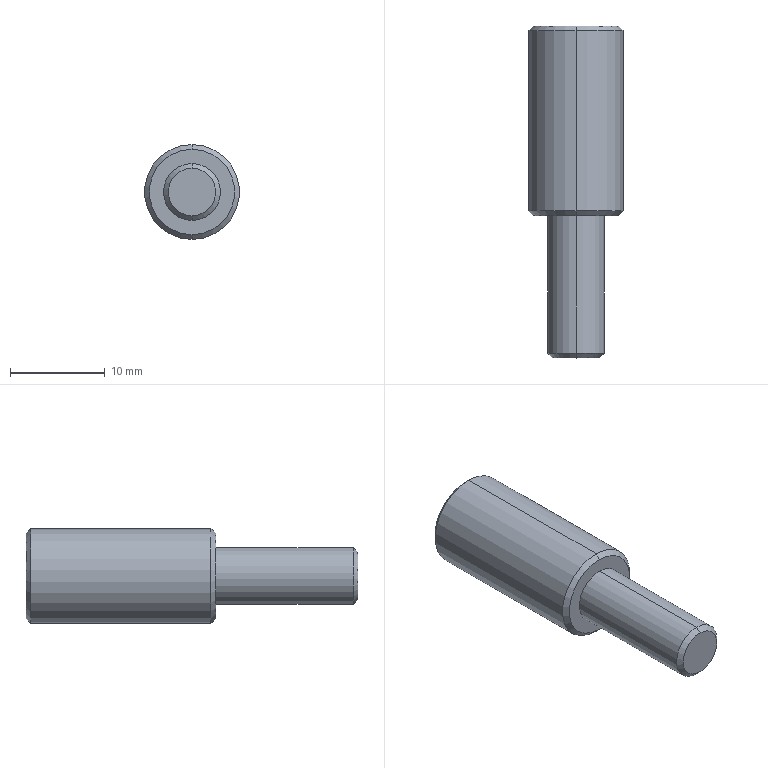Part | SolidWorks | features Chamfer 1, Extrusion 1, ICE 1 | 1 solid | 13 faces | box 10 x 35 x 10 mm | volume 1985 mm3 | cone 6 | cylinder 4 | plane 3 | commonest cylinder face diameters 6 x2 10 x2
STEP:
#1=CARTESIAN_POINT('',(0.,-15.,-2.5));
#2=VERTEX_POINT('',#1);
#3=CARTESIAN_POINT('',(0.,-15.,2.5));
#4=VERTEX_POINT('',#3);
#5=CARTESIAN_POINT('',(0.,-15.,0.));
#6=DIRECTION('',(0.,-1.,0.));
#7=DIRECTION('',(0.,0.,-1.));
#8=AXIS2_PLACEMENT_3D('',#5,#6,#7);
#9=CIRCLE('',#8,2.5);
#10=EDGE_CURVE('',#2,#4,#9,.T.);
#11=ORIENTED_EDGE('',*,*,#10,.F.);
#12=CARTESIAN_POINT('',(0.,-14.5,-3.));
#13=VERTEX_POINT('',#12);
#14=CARTESIAN_POINT('',(0.,-15.,-2.5));
#15=DIRECTION('',(0.,0.7071,-0.7071));
#16=VECTOR('',#15,1000.);
#17=LINE('',#14,#16);
#18=EDGE_CURVE('',#2,#13,#17,.T.);
#19=ORIENTED_EDGE('',*,*,#18,.T.);
#20=CARTESIAN_POINT('',(0.,-14.5,3.));
#21=VERTEX_POINT('',#20);
#22=CARTESIAN_POINT('',(0.,-14.5,0.));
#23=DIRECTION('',(0.,1.,0.));
#24=DIRECTION('',(0.,0.,-1.));
#25=AXIS2_PLACEMENT_3D('',#22,#23,#24);
#26=CIRCLE('',#25,3.);
#27=EDGE_CURVE('',#21,#13,#26,.T.);
#28=ORIENTED_EDGE('',*,*,#27,.F.);
#29=CARTESIAN_POINT('',(0.,-15.,2.5));
#30=DIRECTION('',(0.,0.7071,0.7071));
#31=VECTOR('',#30,1000.);
#32=LINE('',#29,#31);
#33=EDGE_CURVE('',#4,#21,#32,.T.);
#34=ORIENTED_EDGE('',*,*,#33,.F.);
#35=EDGE_LOOP('',(#11,#19,#28,#34));
#36=FACE_OUTER_BOUND('',#35,.T.);
#37=CARTESIAN_POINT('',(0.,-15.,0.));
#38=DIRECTION('',(0.,1.,0.));
#39=DIRECTION('',(0.,0.,1.));
#40=AXIS2_PLACEMENT_3D('',#37,#38,#39);
#41=CONICAL_SURFACE('',#40,2.5,0.7854);
#42=ADVANCED_FACE('',(#36),#41,.T.);
#43=CARTESIAN_POINT('',(0.,0.,-4.5));
#44=VERTEX_POINT('',#43);
#45=CARTESIAN_POINT('',(0.,0.,4.5));
#46=VERTEX_POINT('',#45);
#47=CARTESIAN_POINT('',(0.,0.,0.));
#48=DIRECTION('',(0.,-1.,0.));
#49=DIRECTION('',(0.,0.,1.));
#50=AXIS2_PLACEMENT_3D('',#47,#48,#49);
#51=CIRCLE('',#50,4.5);
#52=EDGE_CURVE('',#44,#46,#51,.T.);
#53=ORIENTED_EDGE('',*,*,#52,.F.);
#54=CARTESIAN_POINT('',(0.,0.5,-5.));
#55=VERTEX_POINT('',#54);
#56=CARTESIAN_POINT('',(0.,0.5,-5.));
#57=DIRECTION('',(0.,0.7071,-0.7071));
#58=VECTOR('',#57,1000.);
#59=LINE('',#56,#58);
#60=EDGE_CURVE('',#44,#55,#59,.T.);
#61=ORIENTED_EDGE('',*,*,#60,.T.);
#62=CARTESIAN_POINT('',(0.,0.5,5.));
#63=VERTEX_POINT('',#62);
#64=CARTESIAN_POINT('',(0.,0.5,0.));
#65=DIRECTION('',(0.,1.,0.));
#66=DIRECTION('',(0.,0.,1.));
#67=AXIS2_PLACEMENT_3D('',#64,#65,#66);
#68=CIRCLE('',#67,5.);
#69=EDGE_CURVE('',#63,#55,#68,.T.);
#70=ORIENTED_EDGE('',*,*,#69,.F.);
#71=CARTESIAN_POINT('',(0.,0.5,5.));
#72=DIRECTION('',(0.,0.7071,0.7071));
#73=VECTOR('',#72,1000.);
#74=LINE('',#71,#73);
#75=EDGE_CURVE('',#46,#63,#74,.T.);
#76=ORIENTED_EDGE('',*,*,#75,.F.);
#77=EDGE_LOOP('',(#53,#61,#70,#76));
#78=FACE_OUTER_BOUND('',#77,.T.);
#79=CARTESIAN_POINT('',(0.,0.5,0.));
#80=DIRECTION('',(0.,1.,0.));
#81=DIRECTION('',(0.,0.,1.));
#82=AXIS2_PLACEMENT_3D('',#79,#80,#81);
#83=CONICAL_SURFACE('',#82,5.,0.7854);
#84=ADVANCED_FACE('',(#78),#83,.T.);
#85=CARTESIAN_POINT('',(0.,20.,4.5));
#86=VERTEX_POINT('',#85);
#87=CARTESIAN_POINT('',(0.,20.,-4.5));
#88=VERTEX_POINT('',#87);
#89=CARTESIAN_POINT('',(0.,20.,0.));
#90=DIRECTION('',(0.,1.,0.));
#91=DIRECTION('',(0.,0.,1.));
#92=AXIS2_PLACEMENT_3D('',#89,#90,#91);
#93=CIRCLE('',#92,4.5);
#94=EDGE_CURVE('',#86,#88,#93,.T.);
#95=ORIENTED_EDGE('',*,*,#94,.F.);
#96=CARTESIAN_POINT('',(0.,19.5,5.));
#97=VERTEX_POINT('',#96);
#98=CARTESIAN_POINT('',(0.,20.,4.5));
#99=DIRECTION('',(0.,-0.7071,0.7071));
#100=VECTOR('',#99,1000.);
#101=LINE('',#98,#100);
#102=EDGE_CURVE('',#86,#97,#101,.T.);
#103=ORIENTED_EDGE('',*,*,#102,.T.);
#104=CARTESIAN_POINT('',(0.,19.5,-5.));
#105=VERTEX_POINT('',#104);
#106=CARTESIAN_POINT('',(0.,19.5,0.));
#107=DIRECTION('',(0.,-1.,0.));
#108=DIRECTION('',(0.,0.,1.));
#109=AXIS2_PLACEMENT_3D('',#106,#107,#108);
#110=CIRCLE('',#109,5.);
#111=EDGE_CURVE('',#105,#97,#110,.T.);
#112=ORIENTED_EDGE('',*,*,#111,.F.);
#113=CARTESIAN_POINT('',(0.,20.,-4.5));
#114=DIRECTION('',(0.,-0.7071,-0.7071));
#115=VECTOR('',#114,1000.);
#116=LINE('',#113,#115);
#117=EDGE_CURVE('',#88,#105,#116,.T.);
#118=ORIENTED_EDGE('',*,*,#117,.F.);
#119=EDGE_LOOP('',(#95,#103,#112,#118));
#120=FACE_OUTER_BOUND('',#119,.T.);
#121=CARTESIAN_POINT('',(0.,20.,0.));
#122=DIRECTION('',(0.,-1.,0.));
#123=DIRECTION('',(0.,0.,-1.));
#124=AXIS2_PLACEMENT_3D('',#121,#122,#123);
#125=CONICAL_SURFACE('',#124,4.5,0.7854);
#126=ADVANCED_FACE('',(#120),#125,.T.);
#127=ORIENTED_EDGE('',*,*,#27,.T.);
#128=CARTESIAN_POINT('',(0.,0.,-3.));
#129=VERTEX_POINT('',#128);
#130=CARTESIAN_POINT('',(0.,-15.,-3.));
#131=DIRECTION('',(0.,1.,0.));
#132=VECTOR('',#131,1000.);
#133=LINE('',#130,#132);
#134=EDGE_CURVE('',#13,#129,#133,.T.);
#135=ORIENTED_EDGE('',*,*,#134,.T.);
#136=CARTESIAN_POINT('',(0.,0.,3.));
#137=VERTEX_POINT('',#136);
#138=CARTESIAN_POINT('',(0.,0.,0.));
#139=DIRECTION('',(0.,-1.,0.));
#140=DIRECTION('',(0.,0.,-1.));
#141=AXIS2_PLACEMENT_3D('',#138,#139,#140);
#142=CIRCLE('',#141,3.);
#143=EDGE_CURVE('',#129,#137,#142,.T.);
#144=ORIENTED_EDGE('',*,*,#143,.T.);
#145=CARTESIAN_POINT('',(0.,-15.,3.));
#146=DIRECTION('',(0.,1.,0.));
#147=VECTOR('',#146,1000.);
#148=LINE('',#145,#147);
#149=EDGE_CURVE('',#21,#137,#148,.T.);
#150=ORIENTED_EDGE('',*,*,#149,.F.);
#151=EDGE_LOOP('',(#127,#135,#144,#150));
#152=FACE_OUTER_BOUND('',#151,.T.);
#153=CARTESIAN_POINT('',(0.,-15.,0.));
#154=DIRECTION('',(0.,1.,0.));
#155=DIRECTION('',(0.,0.,1.));
#156=AXIS2_PLACEMENT_3D('',#153,#154,#155);
#157=CYLINDRICAL_SURFACE('',#156,3.);
#158=ADVANCED_FACE('',(#152),#157,.T.);
#159=ORIENTED_EDGE('',*,*,#111,.T.);
#160=CARTESIAN_POINT('',(0.,20.,5.));
#161=DIRECTION('',(0.,-1.,0.));
#162=VECTOR('',#161,1000.);
#163=LINE('',#160,#162);
#164=EDGE_CURVE('',#97,#63,#163,.T.);
#165=ORIENTED_EDGE('',*,*,#164,.T.);
#166=ORIENTED_EDGE('',*,*,#69,.T.);
#167=CARTESIAN_POINT('',(0.,20.,-5.));
#168=DIRECTION('',(0.,-1.,0.));
#169=VECTOR('',#168,1000.);
#170=LINE('',#167,#169);
#171=EDGE_CURVE('',#105,#55,#170,.T.);
#172=ORIENTED_EDGE('',*,*,#171,.F.);
#173=EDGE_LOOP('',(#159,#165,#166,#172));
#174=FACE_OUTER_BOUND('',#173,.T.);
#175=CARTESIAN_POINT('',(0.,20.,0.));
#176=DIRECTION('',(0.,-1.,0.));
#177=DIRECTION('',(0.,0.,-1.));
#178=AXIS2_PLACEMENT_3D('',#175,#176,#177);
#179=CYLINDRICAL_SURFACE('',#178,5.);
#180=ADVANCED_FACE('',(#174),#179,.T.);
#181=ORIENTED_EDGE('',*,*,#164,.F.);
#182=CARTESIAN_POINT('',(0.,19.5,0.));
#183=DIRECTION('',(0.,-1.,0.));
#184=DIRECTION('',(0.,0.,1.));
#185=AXIS2_PLACEMENT_3D('',#182,#183,#184);
#186=CIRCLE('',#185,5.);
#187=EDGE_CURVE('',#97,#105,#186,.T.);
#188=ORIENTED_EDGE('',*,*,#187,.T.);
#189=ORIENTED_EDGE('',*,*,#171,.T.);
#190=CARTESIAN_POINT('',(0.,0.5,0.));
#191=DIRECTION('',(0.,1.,0.));
#192=DIRECTION('',(0.,0.,1.));
#193=AXIS2_PLACEMENT_3D('',#190,#191,#192);
#194=CIRCLE('',#193,5.);
#195=EDGE_CURVE('',#55,#63,#194,.T.);
#196=ORIENTED_EDGE('',*,*,#195,.T.);
#197=EDGE_LOOP('',(#181,#188,#189,#196));
#198=FACE_OUTER_BOUND('',#197,.T.);
#199=CARTESIAN_POINT('',(0.,20.,0.));
#200=DIRECTION('',(0.,-1.,0.));
#201=DIRECTION('',(0.,0.,-1.));
#202=AXIS2_PLACEMENT_3D('',#199,#200,#201);
#203=CYLINDRICAL_SURFACE('',#202,5.);
#204=ADVANCED_FACE('',(#198),#203,.T.);
#205=CARTESIAN_POINT('',(0.,20.,0.));
#206=DIRECTION('',(0.,1.,0.));
#207=DIRECTION('',(0.,0.,1.));
#208=AXIS2_PLACEMENT_3D('',#205,#206,#207);
#209=CIRCLE('',#208,4.5);
#210=EDGE_CURVE('',#88,#86,#209,.T.);
#211=ORIENTED_EDGE('',*,*,#210,.T.);
#212=ORIENTED_EDGE('',*,*,#94,.T.);
#213=EDGE_LOOP('',(#211,#212));
#214=FACE_OUTER_BOUND('',#213,.T.);
#215=CARTESIAN_POINT('',(0.,20.,0.));
#216=DIRECTION('',(0.,1.,0.));
#217=DIRECTION('',(0.,0.,1.));
#218=AXIS2_PLACEMENT_3D('',#215,#216,#217);
#219=PLANE('',#218);
#220=ADVANCED_FACE('',(#214),#219,.T.);
#221=CARTESIAN_POINT('',(0.,0.,0.));
#222=DIRECTION('',(0.,-1.,0.));
#223=DIRECTION('',(0.,0.,1.));
#224=AXIS2_PLACEMENT_3D('',#221,#222,#223);
#225=CIRCLE('',#224,4.5);
#226=EDGE_CURVE('',#46,#44,#225,.T.);
#227=ORIENTED_EDGE('',*,*,#226,.T.);
#228=ORIENTED_EDGE('',*,*,#52,.T.);
#229=EDGE_LOOP('',(#227,#228));
#230=FACE_OUTER_BOUND('',#229,.T.);
#231=CARTESIAN_POINT('',(0.,0.,0.));
#232=DIRECTION('',(0.,-1.,0.));
#233=DIRECTION('',(0.,0.,-1.));
#234=AXIS2_PLACEMENT_3D('',#231,#232,#233);
#235=CIRCLE('',#234,3.);
#236=EDGE_CURVE('',#137,#129,#235,.T.);
#237=ORIENTED_EDGE('',*,*,#236,.F.);
#238=ORIENTED_EDGE('',*,*,#143,.F.);
#239=EDGE_LOOP('',(#237,#238));
#240=FACE_BOUND('',#239,.T.);
#241=CARTESIAN_POINT('',(0.,0.,0.));
#242=DIRECTION('',(0.,1.,0.));
#243=DIRECTION('',(0.,0.,1.));
#244=AXIS2_PLACEMENT_3D('',#241,#242,#243);
#245=PLANE('',#244);
#246=ADVANCED_FACE('',(#230,#240),#245,.F.);
#247=ORIENTED_EDGE('',*,*,#134,.F.);
#248=CARTESIAN_POINT('',(0.,-14.5,0.));
#249=DIRECTION('',(0.,1.,0.));
#250=DIRECTION('',(0.,0.,-1.));
#251=AXIS2_PLACEMENT_3D('',#248,#249,#250);
#252=CIRCLE('',#251,3.);
#253=EDGE_CURVE('',#13,#21,#252,.T.);
#254=ORIENTED_EDGE('',*,*,#253,.T.);
#255=ORIENTED_EDGE('',*,*,#149,.T.);
#256=ORIENTED_EDGE('',*,*,#236,.T.);
#257=EDGE_LOOP('',(#247,#254,#255,#256));
#258=FACE_OUTER_BOUND('',#257,.T.);
#259=CARTESIAN_POINT('',(0.,-15.,0.));
#260=DIRECTION('',(0.,1.,0.));
#261=DIRECTION('',(0.,0.,1.));
#262=AXIS2_PLACEMENT_3D('',#259,#260,#261);
#263=CYLINDRICAL_SURFACE('',#262,3.);
#264=ADVANCED_FACE('',(#258),#263,.T.);
#265=CARTESIAN_POINT('',(0.,-15.,0.));
#266=DIRECTION('',(0.,-1.,0.));
#267=DIRECTION('',(0.,0.,-1.));
#268=AXIS2_PLACEMENT_3D('',#265,#266,#267);
#269=CIRCLE('',#268,2.5);
#270=EDGE_CURVE('',#4,#2,#269,.T.);
#271=ORIENTED_EDGE('',*,*,#270,.T.);
#272=ORIENTED_EDGE('',*,*,#10,.T.);
#273=EDGE_LOOP('',(#271,#272));
#274=FACE_OUTER_BOUND('',#273,.T.);
#275=CARTESIAN_POINT('',(0.,-15.,0.));
#276=DIRECTION('',(0.,-1.,0.));
#277=DIRECTION('',(0.,0.,-1.));
#278=AXIS2_PLACEMENT_3D('',#275,#276,#277);
#279=PLANE('',#278);
#280=ADVANCED_FACE('',(#274),#279,.T.);
#281=ORIENTED_EDGE('',*,*,#102,.F.);
#282=ORIENTED_EDGE('',*,*,#210,.F.);
#283=ORIENTED_EDGE('',*,*,#117,.T.);
#284=ORIENTED_EDGE('',*,*,#187,.F.);
#285=EDGE_LOOP('',(#281,#282,#283,#284));
#286=FACE_OUTER_BOUND('',#285,.T.);
#287=CARTESIAN_POINT('',(0.,20.,0.));
#288=DIRECTION('',(0.,-1.,0.));
#289=DIRECTION('',(0.,0.,-1.));
#290=AXIS2_PLACEMENT_3D('',#287,#288,#289);
#291=CONICAL_SURFACE('',#290,4.5,0.7854);
#292=ADVANCED_FACE('',(#286),#291,.T.);
#293=ORIENTED_EDGE('',*,*,#60,.F.);
#294=ORIENTED_EDGE('',*,*,#226,.F.);
#295=ORIENTED_EDGE('',*,*,#75,.T.);
#296=ORIENTED_EDGE('',*,*,#195,.F.);
#297=EDGE_LOOP('',(#293,#294,#295,#296));
#298=FACE_OUTER_BOUND('',#297,.T.);
#299=CARTESIAN_POINT('',(0.,0.5,0.));
#300=DIRECTION('',(0.,1.,0.));
#301=DIRECTION('',(0.,0.,1.));
#302=AXIS2_PLACEMENT_3D('',#299,#300,#301);
#303=CONICAL_SURFACE('',#302,5.,0.7854);
#304=ADVANCED_FACE('',(#298),#303,.T.);
#305=ORIENTED_EDGE('',*,*,#18,.F.);
#306=ORIENTED_EDGE('',*,*,#270,.F.);
#307=ORIENTED_EDGE('',*,*,#33,.T.);
#308=ORIENTED_EDGE('',*,*,#253,.F.);
#309=EDGE_LOOP('',(#305,#306,#307,#308));
#310=FACE_OUTER_BOUND('',#309,.T.);
#311=CARTESIAN_POINT('',(0.,-15.,0.));
#312=DIRECTION('',(0.,1.,0.));
#313=DIRECTION('',(0.,0.,1.));
#314=AXIS2_PLACEMENT_3D('',#311,#312,#313);
#315=CONICAL_SURFACE('',#314,2.5,0.7854);
#316=ADVANCED_FACE('',(#310),#315,.T.);
#317=CLOSED_SHELL('',(#42,#84,#126,#158,#180,#204,#220,#246,#264,#280,#292,#304,#316));
#318=MANIFOLD_SOLID_BREP('',#317);
#319=CARTESIAN_POINT('',(0.,0.,0.));
#320=DIRECTION('',(0.,0.,1.));
#321=DIRECTION('',(1.,0.,0.));
#322=AXIS2_PLACEMENT_3D('',#319,#320,#321);
#323=(LENGTH_UNIT()NAMED_UNIT(*)SI_UNIT(.MILLI.,.METRE.));
#324=UNCERTAINTY_MEASURE_WITH_UNIT(LENGTH_MEASURE(0.00001),#323,'','');
#325=(NAMED_UNIT(*)PLANE_ANGLE_UNIT()SI_UNIT($,.RADIAN.));
#326=(NAMED_UNIT(*)SI_UNIT($,.STERADIAN.)SOLID_ANGLE_UNIT());
#327=(GEOMETRIC_REPRESENTATION_CONTEXT(3)GLOBAL_UNCERTAINTY_ASSIGNED_CONTEXT((#324))GLOBAL_UNIT_ASSIGNED_CONTEXT((#323,#325,#326))REPRESENTATION_CONTEXT('',''));
#328=ADVANCED_BREP_SHAPE_REPRESENTATION('',(#318,#322),#327);